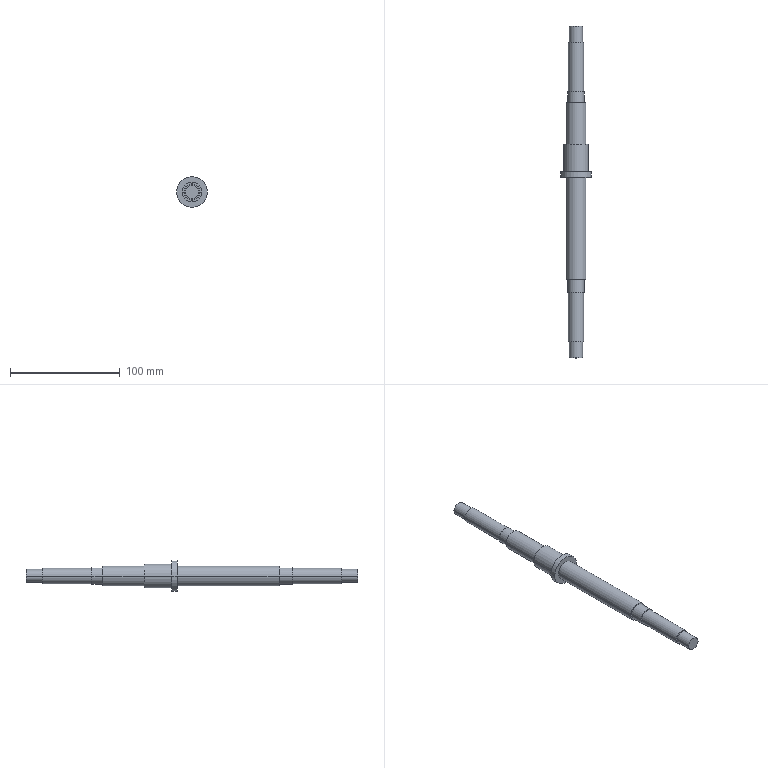Part | SolidWorks | features Revolution 1 | 1 solid | 31 faces | box 28 x 303 x 28 mm | volume 67053 mm3 | cylinder 20 | plane 11 | commonest cylinder face diameters 12 x4 14 x4 15 x4 18 x4 22 x2 28 x2
STEP:
#1=CARTESIAN_POINT('',(-6.,0.,0.));
#2=VERTEX_POINT('',#1);
#3=CARTESIAN_POINT('',(6.,0.,0.));
#4=VERTEX_POINT('',#3);
#5=CARTESIAN_POINT('',(0.,0.,0.));
#6=DIRECTION('',(0.,1.,0.));
#7=DIRECTION('',(-1.,0.,0.));
#8=AXIS2_PLACEMENT_3D('',#5,#6,#7);
#9=CIRCLE('',#8,6.);
#10=EDGE_CURVE('',#2,#4,#9,.T.);
#11=ORIENTED_EDGE('',*,*,#10,.T.);
#12=CARTESIAN_POINT('',(6.,15.,0.));
#13=VERTEX_POINT('',#12);
#14=CARTESIAN_POINT('',(6.,303.,0.));
#15=DIRECTION('',(0.,1.,0.));
#16=VECTOR('',#15,1000.);
#17=LINE('',#14,#16);
#18=EDGE_CURVE('',#4,#13,#17,.T.);
#19=ORIENTED_EDGE('',*,*,#18,.T.);
#20=CARTESIAN_POINT('',(-6.,15.,0.));
#21=VERTEX_POINT('',#20);
#22=CARTESIAN_POINT('',(0.,15.,0.));
#23=DIRECTION('',(0.,1.,0.));
#24=DIRECTION('',(-1.,0.,0.));
#25=AXIS2_PLACEMENT_3D('',#22,#23,#24);
#26=CIRCLE('',#25,6.);
#27=EDGE_CURVE('',#21,#13,#26,.T.);
#28=ORIENTED_EDGE('',*,*,#27,.F.);
#29=CARTESIAN_POINT('',(-6.,303.,0.));
#30=DIRECTION('',(0.,1.,0.));
#31=VECTOR('',#30,1000.);
#32=LINE('',#29,#31);
#33=EDGE_CURVE('',#2,#21,#32,.T.);
#34=ORIENTED_EDGE('',*,*,#33,.F.);
#35=EDGE_LOOP('',(#11,#19,#28,#34));
#36=FACE_OUTER_BOUND('',#35,.T.);
#37=CARTESIAN_POINT('',(0.,303.,0.));
#38=DIRECTION('',(0.,1.,0.));
#39=DIRECTION('',(-1.,0.,0.));
#40=AXIS2_PLACEMENT_3D('',#37,#38,#39);
#41=CYLINDRICAL_SURFACE('',#40,6.);
#42=ADVANCED_FACE('',(#36),#41,.T.);
#43=CARTESIAN_POINT('',(-7.,15.,0.));
#44=VERTEX_POINT('',#43);
#45=CARTESIAN_POINT('',(7.,15.,0.));
#46=VERTEX_POINT('',#45);
#47=CARTESIAN_POINT('',(0.,15.,0.));
#48=DIRECTION('',(0.,1.,0.));
#49=DIRECTION('',(-1.,0.,0.));
#50=AXIS2_PLACEMENT_3D('',#47,#48,#49);
#51=CIRCLE('',#50,7.);
#52=EDGE_CURVE('',#44,#46,#51,.T.);
#53=ORIENTED_EDGE('',*,*,#52,.T.);
#54=CARTESIAN_POINT('',(7.,60.,0.));
#55=VERTEX_POINT('',#54);
#56=CARTESIAN_POINT('',(7.,303.,0.));
#57=DIRECTION('',(0.,1.,0.));
#58=VECTOR('',#57,1000.);
#59=LINE('',#56,#58);
#60=EDGE_CURVE('',#46,#55,#59,.T.);
#61=ORIENTED_EDGE('',*,*,#60,.T.);
#62=CARTESIAN_POINT('',(-7.,60.,0.));
#63=VERTEX_POINT('',#62);
#64=CARTESIAN_POINT('',(0.,60.,0.));
#65=DIRECTION('',(0.,1.,0.));
#66=DIRECTION('',(-1.,0.,0.));
#67=AXIS2_PLACEMENT_3D('',#64,#65,#66);
#68=CIRCLE('',#67,7.);
#69=EDGE_CURVE('',#63,#55,#68,.T.);
#70=ORIENTED_EDGE('',*,*,#69,.F.);
#71=CARTESIAN_POINT('',(-7.,303.,0.));
#72=DIRECTION('',(0.,1.,0.));
#73=VECTOR('',#72,1000.);
#74=LINE('',#71,#73);
#75=EDGE_CURVE('',#44,#63,#74,.T.);
#76=ORIENTED_EDGE('',*,*,#75,.F.);
#77=EDGE_LOOP('',(#53,#61,#70,#76));
#78=FACE_OUTER_BOUND('',#77,.T.);
#79=CARTESIAN_POINT('',(0.,303.,0.));
#80=DIRECTION('',(0.,1.,0.));
#81=DIRECTION('',(-1.,0.,0.));
#82=AXIS2_PLACEMENT_3D('',#79,#80,#81);
#83=CYLINDRICAL_SURFACE('',#82,7.);
#84=ADVANCED_FACE('',(#78),#83,.T.);
#85=CARTESIAN_POINT('',(-7.5,60.,0.));
#86=VERTEX_POINT('',#85);
#87=CARTESIAN_POINT('',(7.5,60.,0.));
#88=VERTEX_POINT('',#87);
#89=CARTESIAN_POINT('',(0.,60.,0.));
#90=DIRECTION('',(0.,1.,0.));
#91=DIRECTION('',(-1.,0.,0.));
#92=AXIS2_PLACEMENT_3D('',#89,#90,#91);
#93=CIRCLE('',#92,7.5);
#94=EDGE_CURVE('',#86,#88,#93,.T.);
#95=ORIENTED_EDGE('',*,*,#94,.T.);
#96=CARTESIAN_POINT('',(7.5,72.,0.));
#97=VERTEX_POINT('',#96);
#98=CARTESIAN_POINT('',(7.5,303.,0.));
#99=DIRECTION('',(0.,1.,0.));
#100=VECTOR('',#99,1000.);
#101=LINE('',#98,#100);
#102=EDGE_CURVE('',#88,#97,#101,.T.);
#103=ORIENTED_EDGE('',*,*,#102,.T.);
#104=CARTESIAN_POINT('',(-7.5,72.,0.));
#105=VERTEX_POINT('',#104);
#106=CARTESIAN_POINT('',(0.,72.,0.));
#107=DIRECTION('',(0.,1.,0.));
#108=DIRECTION('',(-1.,0.,0.));
#109=AXIS2_PLACEMENT_3D('',#106,#107,#108);
#110=CIRCLE('',#109,7.5);
#111=EDGE_CURVE('',#105,#97,#110,.T.);
#112=ORIENTED_EDGE('',*,*,#111,.F.);
#113=CARTESIAN_POINT('',(-7.5,303.,0.));
#114=DIRECTION('',(0.,1.,0.));
#115=VECTOR('',#114,1000.);
#116=LINE('',#113,#115);
#117=EDGE_CURVE('',#86,#105,#116,.T.);
#118=ORIENTED_EDGE('',*,*,#117,.F.);
#119=EDGE_LOOP('',(#95,#103,#112,#118));
#120=FACE_OUTER_BOUND('',#119,.T.);
#121=CARTESIAN_POINT('',(0.,303.,0.));
#122=DIRECTION('',(0.,1.,0.));
#123=DIRECTION('',(-1.,0.,0.));
#124=AXIS2_PLACEMENT_3D('',#121,#122,#123);
#125=CYLINDRICAL_SURFACE('',#124,7.5);
#126=ADVANCED_FACE('',(#120),#125,.T.);
#127=CARTESIAN_POINT('',(-9.,72.,0.));
#128=VERTEX_POINT('',#127);
#129=CARTESIAN_POINT('',(9.,72.,0.));
#130=VERTEX_POINT('',#129);
#131=CARTESIAN_POINT('',(0.,72.,0.));
#132=DIRECTION('',(0.,1.,0.));
#133=DIRECTION('',(-1.,0.,0.));
#134=AXIS2_PLACEMENT_3D('',#131,#132,#133);
#135=CIRCLE('',#134,9.);
#136=EDGE_CURVE('',#128,#130,#135,.T.);
#137=ORIENTED_EDGE('',*,*,#136,.T.);
#138=CARTESIAN_POINT('',(9.,165.,0.));
#139=VERTEX_POINT('',#138);
#140=CARTESIAN_POINT('',(9.,303.,0.));
#141=DIRECTION('',(0.,1.,0.));
#142=VECTOR('',#141,1000.);
#143=LINE('',#140,#142);
#144=EDGE_CURVE('',#130,#139,#143,.T.);
#145=ORIENTED_EDGE('',*,*,#144,.T.);
#146=CARTESIAN_POINT('',(-9.,165.,0.));
#147=VERTEX_POINT('',#146);
#148=CARTESIAN_POINT('',(0.,165.,0.));
#149=DIRECTION('',(0.,1.,0.));
#150=DIRECTION('',(-1.,0.,0.));
#151=AXIS2_PLACEMENT_3D('',#148,#149,#150);
#152=CIRCLE('',#151,9.);
#153=EDGE_CURVE('',#147,#139,#152,.T.);
#154=ORIENTED_EDGE('',*,*,#153,.F.);
#155=CARTESIAN_POINT('',(-9.,303.,0.));
#156=DIRECTION('',(0.,1.,0.));
#157=VECTOR('',#156,1000.);
#158=LINE('',#155,#157);
#159=EDGE_CURVE('',#128,#147,#158,.T.);
#160=ORIENTED_EDGE('',*,*,#159,.F.);
#161=EDGE_LOOP('',(#137,#145,#154,#160));
#162=FACE_OUTER_BOUND('',#161,.T.);
#163=CARTESIAN_POINT('',(0.,303.,0.));
#164=DIRECTION('',(0.,1.,0.));
#165=DIRECTION('',(-1.,0.,0.));
#166=AXIS2_PLACEMENT_3D('',#163,#164,#165);
#167=CYLINDRICAL_SURFACE('',#166,9.);
#168=ADVANCED_FACE('',(#162),#167,.T.);
#169=CARTESIAN_POINT('',(-14.,165.,0.));
#170=VERTEX_POINT('',#169);
#171=CARTESIAN_POINT('',(14.,165.,0.));
#172=VERTEX_POINT('',#171);
#173=CARTESIAN_POINT('',(0.,165.,0.));
#174=DIRECTION('',(0.,1.,0.));
#175=DIRECTION('',(-1.,0.,0.));
#176=AXIS2_PLACEMENT_3D('',#173,#174,#175);
#177=CIRCLE('',#176,14.);
#178=EDGE_CURVE('',#170,#172,#177,.T.);
#179=ORIENTED_EDGE('',*,*,#178,.T.);
#180=CARTESIAN_POINT('',(14.,170.,0.));
#181=VERTEX_POINT('',#180);
#182=CARTESIAN_POINT('',(14.,303.,0.));
#183=DIRECTION('',(0.,1.,0.));
#184=VECTOR('',#183,1000.);
#185=LINE('',#182,#184);
#186=EDGE_CURVE('',#172,#181,#185,.T.);
#187=ORIENTED_EDGE('',*,*,#186,.T.);
#188=CARTESIAN_POINT('',(-14.,170.,0.));
#189=VERTEX_POINT('',#188);
#190=CARTESIAN_POINT('',(0.,170.,0.));
#191=DIRECTION('',(0.,1.,0.));
#192=DIRECTION('',(-1.,0.,0.));
#193=AXIS2_PLACEMENT_3D('',#190,#191,#192);
#194=CIRCLE('',#193,14.);
#195=EDGE_CURVE('',#189,#181,#194,.T.);
#196=ORIENTED_EDGE('',*,*,#195,.F.);
#197=CARTESIAN_POINT('',(-14.,303.,0.));
#198=DIRECTION('',(0.,1.,0.));
#199=VECTOR('',#198,1000.);
#200=LINE('',#197,#199);
#201=EDGE_CURVE('',#170,#189,#200,.T.);
#202=ORIENTED_EDGE('',*,*,#201,.F.);
#203=EDGE_LOOP('',(#179,#187,#196,#202));
#204=FACE_OUTER_BOUND('',#203,.T.);
#205=CARTESIAN_POINT('',(0.,303.,0.));
#206=DIRECTION('',(0.,1.,0.));
#207=DIRECTION('',(-1.,0.,0.));
#208=AXIS2_PLACEMENT_3D('',#205,#206,#207);
#209=CYLINDRICAL_SURFACE('',#208,14.);
#210=ADVANCED_FACE('',(#204),#209,.T.);
#211=CARTESIAN_POINT('',(-11.,170.,0.));
#212=VERTEX_POINT('',#211);
#213=CARTESIAN_POINT('',(11.,170.,0.));
#214=VERTEX_POINT('',#213);
#215=CARTESIAN_POINT('',(0.,170.,0.));
#216=DIRECTION('',(0.,1.,0.));
#217=DIRECTION('',(-1.,0.,0.));
#218=AXIS2_PLACEMENT_3D('',#215,#216,#217);
#219=CIRCLE('',#218,11.);
#220=EDGE_CURVE('',#212,#214,#219,.T.);
#221=ORIENTED_EDGE('',*,*,#220,.T.);
#222=CARTESIAN_POINT('',(11.,195.,0.));
#223=VERTEX_POINT('',#222);
#224=CARTESIAN_POINT('',(11.,303.,0.));
#225=DIRECTION('',(0.,1.,0.));
#226=VECTOR('',#225,1000.);
#227=LINE('',#224,#226);
#228=EDGE_CURVE('',#214,#223,#227,.T.);
#229=ORIENTED_EDGE('',*,*,#228,.T.);
#230=CARTESIAN_POINT('',(-11.,195.,0.));
#231=VERTEX_POINT('',#230);
#232=CARTESIAN_POINT('',(0.,195.,0.));
#233=DIRECTION('',(0.,1.,0.));
#234=DIRECTION('',(-1.,0.,0.));
#235=AXIS2_PLACEMENT_3D('',#232,#233,#234);
#236=CIRCLE('',#235,11.);
#237=EDGE_CURVE('',#231,#223,#236,.T.);
#238=ORIENTED_EDGE('',*,*,#237,.F.);
#239=CARTESIAN_POINT('',(-11.,303.,0.));
#240=DIRECTION('',(0.,1.,0.));
#241=VECTOR('',#240,1000.);
#242=LINE('',#239,#241);
#243=EDGE_CURVE('',#212,#231,#242,.T.);
#244=ORIENTED_EDGE('',*,*,#243,.F.);
#245=EDGE_LOOP('',(#221,#229,#238,#244));
#246=FACE_OUTER_BOUND('',#245,.T.);
#247=CARTESIAN_POINT('',(0.,303.,0.));
#248=DIRECTION('',(0.,1.,0.));
#249=DIRECTION('',(-1.,0.,0.));
#250=AXIS2_PLACEMENT_3D('',#247,#248,#249);
#251=CYLINDRICAL_SURFACE('',#250,11.);
#252=ADVANCED_FACE('',(#246),#251,.T.);
#253=CARTESIAN_POINT('',(-9.,195.,0.));
#254=VERTEX_POINT('',#253);
#255=CARTESIAN_POINT('',(9.,195.,0.));
#256=VERTEX_POINT('',#255);
#257=CARTESIAN_POINT('',(0.,195.,0.));
#258=DIRECTION('',(0.,1.,0.));
#259=DIRECTION('',(-1.,0.,0.));
#260=AXIS2_PLACEMENT_3D('',#257,#258,#259);
#261=CIRCLE('',#260,9.);
#262=EDGE_CURVE('',#254,#256,#261,.T.);
#263=ORIENTED_EDGE('',*,*,#262,.T.);
#264=CARTESIAN_POINT('',(9.,233.,0.));
#265=VERTEX_POINT('',#264);
#266=CARTESIAN_POINT('',(9.,303.,0.));
#267=DIRECTION('',(0.,1.,0.));
#268=VECTOR('',#267,1000.);
#269=LINE('',#266,#268);
#270=EDGE_CURVE('',#256,#265,#269,.T.);
#271=ORIENTED_EDGE('',*,*,#270,.T.);
#272=CARTESIAN_POINT('',(-9.,233.,0.));
#273=VERTEX_POINT('',#272);
#274=CARTESIAN_POINT('',(0.,233.,0.));
#275=DIRECTION('',(0.,1.,0.));
#276=DIRECTION('',(-1.,0.,0.));
#277=AXIS2_PLACEMENT_3D('',#274,#275,#276);
#278=CIRCLE('',#277,9.);
#279=EDGE_CURVE('',#273,#265,#278,.T.);
#280=ORIENTED_EDGE('',*,*,#279,.F.);
#281=CARTESIAN_POINT('',(-9.,303.,0.));
#282=DIRECTION('',(0.,1.,0.));
#283=VECTOR('',#282,1000.);
#284=LINE('',#281,#283);
#285=EDGE_CURVE('',#254,#273,#284,.T.);
#286=ORIENTED_EDGE('',*,*,#285,.F.);
#287=EDGE_LOOP('',(#263,#271,#280,#286));
#288=FACE_OUTER_BOUND('',#287,.T.);
#289=CARTESIAN_POINT('',(0.,303.,0.));
#290=DIRECTION('',(0.,1.,0.));
#291=DIRECTION('',(-1.,0.,0.));
#292=AXIS2_PLACEMENT_3D('',#289,#290,#291);
#293=CYLINDRICAL_SURFACE('',#292,9.);
#294=ADVANCED_FACE('',(#288),#293,.T.);
#295=CARTESIAN_POINT('',(-7.5,233.,0.));
#296=VERTEX_POINT('',#295);
#297=CARTESIAN_POINT('',(7.5,233.,0.));
#298=VERTEX_POINT('',#297);
#299=CARTESIAN_POINT('',(0.,233.,0.));
#300=DIRECTION('',(0.,1.,0.));
#301=DIRECTION('',(-1.,0.,0.));
#302=AXIS2_PLACEMENT_3D('',#299,#300,#301);
#303=CIRCLE('',#302,7.5);
#304=EDGE_CURVE('',#296,#298,#303,.T.);
#305=ORIENTED_EDGE('',*,*,#304,.T.);
#306=CARTESIAN_POINT('',(7.5,243.,0.));
#307=VERTEX_POINT('',#306);
#308=CARTESIAN_POINT('',(7.5,303.,0.));
#309=DIRECTION('',(0.,1.,0.));
#310=VECTOR('',#309,1000.);
#311=LINE('',#308,#310);
#312=EDGE_CURVE('',#298,#307,#311,.T.);
#313=ORIENTED_EDGE('',*,*,#312,.T.);
#314=CARTESIAN_POINT('',(-7.5,243.,0.));
#315=VERTEX_POINT('',#314);
#316=CARTESIAN_POINT('',(0.,243.,0.));
#317=DIRECTION('',(0.,1.,0.));
#318=DIRECTION('',(-1.,0.,0.));
#319=AXIS2_PLACEMENT_3D('',#316,#317,#318);
#320=CIRCLE('',#319,7.5);
#321=EDGE_CURVE('',#315,#307,#320,.T.);
#322=ORIENTED_EDGE('',*,*,#321,.F.);
#323=CARTESIAN_POINT('',(-7.5,303.,0.));
#324=DIRECTION('',(0.,1.,0.));
#325=VECTOR('',#324,1000.);
#326=LINE('',#323,#325);
#327=EDGE_CURVE('',#296,#315,#326,.T.);
#328=ORIENTED_EDGE('',*,*,#327,.F.);
#329=EDGE_LOOP('',(#305,#313,#322,#328));
#330=FACE_OUTER_BOUND('',#329,.T.);
#331=CARTESIAN_POINT('',(0.,303.,0.));
#332=DIRECTION('',(0.,1.,0.));
#333=DIRECTION('',(-1.,0.,0.));
#334=AXIS2_PLACEMENT_3D('',#331,#332,#333);
#335=CYLINDRICAL_SURFACE('',#334,7.5);
#336=ADVANCED_FACE('',(#330),#335,.T.);
#337=CARTESIAN_POINT('',(-7.,243.,0.));
#338=VERTEX_POINT('',#337);
#339=CARTESIAN_POINT('',(7.,243.,0.));
#340=VERTEX_POINT('',#339);
#341=CARTESIAN_POINT('',(0.,243.,0.));
#342=DIRECTION('',(0.,1.,0.));
#343=DIRECTION('',(-1.,0.,0.));
#344=AXIS2_PLACEMENT_3D('',#341,#342,#343);
#345=CIRCLE('',#344,7.);
#346=EDGE_CURVE('',#338,#340,#345,.T.);
#347=ORIENTED_EDGE('',*,*,#346,.T.);
#348=CARTESIAN_POINT('',(7.,288.,0.));
#349=VERTEX_POINT('',#348);
#350=CARTESIAN_POINT('',(7.,303.,0.));
#351=DIRECTION('',(0.,1.,0.));
#352=VECTOR('',#351,1000.);
#353=LINE('',#350,#352);
#354=EDGE_CURVE('',#340,#349,#353,.T.);
#355=ORIENTED_EDGE('',*,*,#354,.T.);
#356=CARTESIAN_POINT('',(-7.,288.,0.));
#357=VERTEX_POINT('',#356);
#358=CARTESIAN_POINT('',(0.,288.,0.));
#359=DIRECTION('',(0.,1.,0.));
#360=DIRECTION('',(-1.,0.,0.));
#361=AXIS2_PLACEMENT_3D('',#358,#359,#360);
#362=CIRCLE('',#361,7.);
#363=EDGE_CURVE('',#357,#349,#362,.T.);
#364=ORIENTED_EDGE('',*,*,#363,.F.);
#365=CARTESIAN_POINT('',(-7.,303.,0.));
#366=DIRECTION('',(0.,1.,0.));
#367=VECTOR('',#366,1000.);
#368=LINE('',#365,#367);
#369=EDGE_CURVE('',#338,#357,#368,.T.);
#370=ORIENTED_EDGE('',*,*,#369,.F.);
#371=EDGE_LOOP('',(#347,#355,#364,#370));
#372=FACE_OUTER_BOUND('',#371,.T.);
#373=CARTESIAN_POINT('',(0.,303.,0.));
#374=DIRECTION('',(0.,1.,0.));
#375=DIRECTION('',(-1.,0.,0.));
#376=AXIS2_PLACEMENT_3D('',#373,#374,#375);
#377=CYLINDRICAL_SURFACE('',#376,7.);
#378=ADVANCED_FACE('',(#372),#377,.T.);
#379=CARTESIAN_POINT('',(-6.,288.,0.));
#380=VERTEX_POINT('',#379);
#381=CARTESIAN_POINT('',(6.,288.,0.));
#382=VERTEX_POINT('',#381);
#383=CARTESIAN_POINT('',(0.,288.,0.));
#384=DIRECTION('',(0.,1.,0.));
#385=DIRECTION('',(-1.,0.,0.));
#386=AXIS2_PLACEMENT_3D('',#383,#384,#385);
#387=CIRCLE('',#386,6.);
#388=EDGE_CURVE('',#380,#382,#387,.T.);
#389=ORIENTED_EDGE('',*,*,#388,.T.);
#390=CARTESIAN_POINT('',(6.,303.,0.));
#391=VERTEX_POINT('',#390);
#392=CARTESIAN_POINT('',(6.,303.,0.));
#393=DIRECTION('',(0.,1.,0.));
#394=VECTOR('',#393,1000.);
#395=LINE('',#392,#394);
#396=EDGE_CURVE('',#382,#391,#395,.T.);
#397=ORIENTED_EDGE('',*,*,#396,.T.);
#398=CARTESIAN_POINT('',(-6.,303.,0.));
#399=VERTEX_POINT('',#398);
#400=CARTESIAN_POINT('',(0.,303.,0.));
#401=DIRECTION('',(0.,1.,0.));
#402=DIRECTION('',(-1.,0.,0.));
#403=AXIS2_PLACEMENT_3D('',#400,#401,#402);
#404=CIRCLE('',#403,6.);
#405=EDGE_CURVE('',#399,#391,#404,.T.);
#406=ORIENTED_EDGE('',*,*,#405,.F.);
#407=CARTESIAN_POINT('',(-6.,303.,0.));
#408=DIRECTION('',(0.,1.,0.));
#409=VECTOR('',#408,1000.);
#410=LINE('',#407,#409);
#411=EDGE_CURVE('',#380,#399,#410,.T.);
#412=ORIENTED_EDGE('',*,*,#411,.F.);
#413=EDGE_LOOP('',(#389,#397,#406,#412));
#414=FACE_OUTER_BOUND('',#413,.T.);
#415=CARTESIAN_POINT('',(0.,303.,0.));
#416=DIRECTION('',(0.,1.,0.));
#417=DIRECTION('',(-1.,0.,0.));
#418=AXIS2_PLACEMENT_3D('',#415,#416,#417);
#419=CYLINDRICAL_SURFACE('',#418,6.);
#420=ADVANCED_FACE('',(#414),#419,.T.);
#421=ORIENTED_EDGE('',*,*,#405,.T.);
#422=CARTESIAN_POINT('',(0.,303.,0.));
#423=DIRECTION('',(0.,1.,0.));
#424=DIRECTION('',(-1.,0.,0.));
#425=AXIS2_PLACEMENT_3D('',#422,#423,#424);
#426=CIRCLE('',#425,6.);
#427=EDGE_CURVE('',#391,#399,#426,.T.);
#428=ORIENTED_EDGE('',*,*,#427,.T.);
#429=EDGE_LOOP('',(#421,#428));
#430=FACE_OUTER_BOUND('',#429,.T.);
#431=CARTESIAN_POINT('',(0.,303.,0.));
#432=DIRECTION('',(0.,1.,0.));
#433=DIRECTION('',(-1.,0.,0.));
#434=AXIS2_PLACEMENT_3D('',#431,#432,#433);
#435=PLANE('',#434);
#436=ADVANCED_FACE('',(#430),#435,.T.);
#437=ORIENTED_EDGE('',*,*,#396,.F.);
#438=CARTESIAN_POINT('',(0.,288.,0.));
#439=DIRECTION('',(0.,1.,0.));
#440=DIRECTION('',(-1.,0.,0.));
#441=AXIS2_PLACEMENT_3D('',#438,#439,#440);
#442=CIRCLE('',#441,6.);
#443=EDGE_CURVE('',#382,#380,#442,.T.);
#444=ORIENTED_EDGE('',*,*,#443,.T.);
#445=ORIENTED_EDGE('',*,*,#411,.T.);
#446=ORIENTED_EDGE('',*,*,#427,.F.);
#447=EDGE_LOOP('',(#437,#444,#445,#446));
#448=FACE_OUTER_BOUND('',#447,.T.);
#449=CARTESIAN_POINT('',(0.,303.,0.));
#450=DIRECTION('',(0.,1.,0.));
#451=DIRECTION('',(-1.,0.,0.));
#452=AXIS2_PLACEMENT_3D('',#449,#450,#451);
#453=CYLINDRICAL_SURFACE('',#452,6.);
#454=ADVANCED_FACE('',(#448),#453,.T.);
#455=ORIENTED_EDGE('',*,*,#363,.T.);
#456=CARTESIAN_POINT('',(0.,288.,0.));
#457=DIRECTION('',(0.,1.,0.));
#458=DIRECTION('',(-1.,0.,0.));
#459=AXIS2_PLACEMENT_3D('',#456,#457,#458);
#460=CIRCLE('',#459,7.);
#461=EDGE_CURVE('',#349,#357,#460,.T.);
#462=ORIENTED_EDGE('',*,*,#461,.T.);
#463=EDGE_LOOP('',(#455,#462));
#464=FACE_OUTER_BOUND('',#463,.T.);
#465=ORIENTED_EDGE('',*,*,#388,.F.);
#466=ORIENTED_EDGE('',*,*,#443,.F.);
#467=EDGE_LOOP('',(#465,#466));
#468=FACE_BOUND('',#467,.T.);
#469=CARTESIAN_POINT('',(-6.,288.,0.));
#470=DIRECTION('',(0.,1.,0.));
#471=DIRECTION('',(-1.,0.,0.));
#472=AXIS2_PLACEMENT_3D('',#469,#470,#471);
#473=PLANE('',#472);
#474=ADVANCED_FACE('',(#464,#468),#473,.T.);
#475=ORIENTED_EDGE('',*,*,#354,.F.);
#476=CARTESIAN_POINT('',(0.,243.,0.));
#477=DIRECTION('',(0.,1.,0.));
#478=DIRECTION('',(-1.,0.,0.));
#479=AXIS2_PLACEMENT_3D('',#476,#477,#478);
#480=CIRCLE('',#479,7.);
#481=EDGE_CURVE('',#340,#338,#480,.T.);
#482=ORIENTED_EDGE('',*,*,#481,.T.);
#483=ORIENTED_EDGE('',*,*,#369,.T.);
#484=ORIENTED_EDGE('',*,*,#461,.F.);
#485=EDGE_LOOP('',(#475,#482,#483,#484));
#486=FACE_OUTER_BOUND('',#485,.T.);
#487=CARTESIAN_POINT('',(0.,303.,0.));
#488=DIRECTION('',(0.,1.,0.));
#489=DIRECTION('',(-1.,0.,0.));
#490=AXIS2_PLACEMENT_3D('',#487,#488,#489);
#491=CYLINDRICAL_SURFACE('',#490,7.);
#492=ADVANCED_FACE('',(#486),#491,.T.);
#493=ORIENTED_EDGE('',*,*,#321,.T.);
#494=CARTESIAN_POINT('',(0.,243.,0.));
#495=DIRECTION('',(0.,1.,0.));
#496=DIRECTION('',(-1.,0.,0.));
#497=AXIS2_PLACEMENT_3D('',#494,#495,#496);
#498=CIRCLE('',#497,7.5);
#499=EDGE_CURVE('',#307,#315,#498,.T.);
#500=ORIENTED_EDGE('',*,*,#499,.T.);
#501=EDGE_LOOP('',(#493,#500));
#502=FACE_OUTER_BOUND('',#501,.T.);
#503=ORIENTED_EDGE('',*,*,#346,.F.);
#504=ORIENTED_EDGE('',*,*,#481,.F.);
#505=EDGE_LOOP('',(#503,#504));
#506=FACE_BOUND('',#505,.T.);
#507=CARTESIAN_POINT('',(-7.,243.,0.));
#508=DIRECTION('',(0.,1.,0.));
#509=DIRECTION('',(-1.,0.,0.));
#510=AXIS2_PLACEMENT_3D('',#507,#508,#509);
#511=PLANE('',#510);
#512=ADVANCED_FACE('',(#502,#506),#511,.T.);
#513=ORIENTED_EDGE('',*,*,#312,.F.);
#514=CARTESIAN_POINT('',(0.,233.,0.));
#515=DIRECTION('',(0.,1.,0.));
#516=DIRECTION('',(-1.,0.,0.));
#517=AXIS2_PLACEMENT_3D('',#514,#515,#516);
#518=CIRCLE('',#517,7.5);
#519=EDGE_CURVE('',#298,#296,#518,.T.);
#520=ORIENTED_EDGE('',*,*,#519,.T.);
#521=ORIENTED_EDGE('',*,*,#327,.T.);
#522=ORIENTED_EDGE('',*,*,#499,.F.);
#523=EDGE_LOOP('',(#513,#520,#521,#522));
#524=FACE_OUTER_BOUND('',#523,.T.);
#525=CARTESIAN_POINT('',(0.,303.,0.));
#526=DIRECTION('',(0.,1.,0.));
#527=DIRECTION('',(-1.,0.,0.));
#528=AXIS2_PLACEMENT_3D('',#525,#526,#527);
#529=CYLINDRICAL_SURFACE('',#528,7.5);
#530=ADVANCED_FACE('',(#524),#529,.T.);
#531=ORIENTED_EDGE('',*,*,#279,.T.);
#532=CARTESIAN_POINT('',(0.,233.,0.));
#533=DIRECTION('',(0.,1.,0.));
#534=DIRECTION('',(-1.,0.,0.));
#535=AXIS2_PLACEMENT_3D('',#532,#533,#534);
#536=CIRCLE('',#535,9.);
#537=EDGE_CURVE('',#265,#273,#536,.T.);
#538=ORIENTED_EDGE('',*,*,#537,.T.);
#539=EDGE_LOOP('',(#531,#538));
#540=FACE_OUTER_BOUND('',#539,.T.);
#541=ORIENTED_EDGE('',*,*,#304,.F.);
#542=ORIENTED_EDGE('',*,*,#519,.F.);
#543=EDGE_LOOP('',(#541,#542));
#544=FACE_BOUND('',#543,.T.);
#545=CARTESIAN_POINT('',(-7.5,233.,0.));
#546=DIRECTION('',(0.,1.,0.));
#547=DIRECTION('',(-1.,0.,0.));
#548=AXIS2_PLACEMENT_3D('',#545,#546,#547);
#549=PLANE('',#548);
#550=ADVANCED_FACE('',(#540,#544),#549,.T.);
#551=ORIENTED_EDGE('',*,*,#270,.F.);
#552=CARTESIAN_POINT('',(0.,195.,0.));
#553=DIRECTION('',(0.,1.,0.));
#554=DIRECTION('',(-1.,0.,0.));
#555=AXIS2_PLACEMENT_3D('',#552,#553,#554);
#556=CIRCLE('',#555,9.);
#557=EDGE_CURVE('',#256,#254,#556,.T.);
#558=ORIENTED_EDGE('',*,*,#557,.T.);
#559=ORIENTED_EDGE('',*,*,#285,.T.);
#560=ORIENTED_EDGE('',*,*,#537,.F.);
#561=EDGE_LOOP('',(#551,#558,#559,#560));
#562=FACE_OUTER_BOUND('',#561,.T.);
#563=CARTESIAN_POINT('',(0.,303.,0.));
#564=DIRECTION('',(0.,1.,0.));
#565=DIRECTION('',(-1.,0.,0.));
#566=AXIS2_PLACEMENT_3D('',#563,#564,#565);
#567=CYLINDRICAL_SURFACE('',#566,9.);
#568=ADVANCED_FACE('',(#562),#567,.T.);
#569=ORIENTED_EDGE('',*,*,#237,.T.);
#570=CARTESIAN_POINT('',(0.,195.,0.));
#571=DIRECTION('',(0.,1.,0.));
#572=DIRECTION('',(-1.,0.,0.));
#573=AXIS2_PLACEMENT_3D('',#570,#571,#572);
#574=CIRCLE('',#573,11.);
#575=EDGE_CURVE('',#223,#231,#574,.T.);
#576=ORIENTED_EDGE('',*,*,#575,.T.);
#577=EDGE_LOOP('',(#569,#576));
#578=FACE_OUTER_BOUND('',#577,.T.);
#579=ORIENTED_EDGE('',*,*,#262,.F.);
#580=ORIENTED_EDGE('',*,*,#557,.F.);
#581=EDGE_LOOP('',(#579,#580));
#582=FACE_BOUND('',#581,.T.);
#583=CARTESIAN_POINT('',(-9.,195.,0.));
#584=DIRECTION('',(0.,1.,0.));
#585=DIRECTION('',(-1.,0.,0.));
#586=AXIS2_PLACEMENT_3D('',#583,#584,#585);
#587=PLANE('',#586);
#588=ADVANCED_FACE('',(#578,#582),#587,.T.);
#589=ORIENTED_EDGE('',*,*,#228,.F.);
#590=CARTESIAN_POINT('',(0.,170.,0.));
#591=DIRECTION('',(0.,1.,0.));
#592=DIRECTION('',(-1.,0.,0.));
#593=AXIS2_PLACEMENT_3D('',#590,#591,#592);
#594=CIRCLE('',#593,11.);
#595=EDGE_CURVE('',#214,#212,#594,.T.);
#596=ORIENTED_EDGE('',*,*,#595,.T.);
#597=ORIENTED_EDGE('',*,*,#243,.T.);
#598=ORIENTED_EDGE('',*,*,#575,.F.);
#599=EDGE_LOOP('',(#589,#596,#597,#598));
#600=FACE_OUTER_BOUND('',#599,.T.);
#601=CARTESIAN_POINT('',(0.,303.,0.));
#602=DIRECTION('',(0.,1.,0.));
#603=DIRECTION('',(-1.,0.,0.));
#604=AXIS2_PLACEMENT_3D('',#601,#602,#603);
#605=CYLINDRICAL_SURFACE('',#604,11.);
#606=ADVANCED_FACE('',(#600),#605,.T.);
#607=ORIENTED_EDGE('',*,*,#195,.T.);
#608=CARTESIAN_POINT('',(0.,170.,0.));
#609=DIRECTION('',(0.,1.,0.));
#610=DIRECTION('',(-1.,0.,0.));
#611=AXIS2_PLACEMENT_3D('',#608,#609,#610);
#612=CIRCLE('',#611,14.);
#613=EDGE_CURVE('',#181,#189,#612,.T.);
#614=ORIENTED_EDGE('',*,*,#613,.T.);
#615=EDGE_LOOP('',(#607,#614));
#616=FACE_OUTER_BOUND('',#615,.T.);
#617=ORIENTED_EDGE('',*,*,#220,.F.);
#618=ORIENTED_EDGE('',*,*,#595,.F.);
#619=EDGE_LOOP('',(#617,#618));
#620=FACE_BOUND('',#619,.T.);
#621=CARTESIAN_POINT('',(-11.,170.,0.));
#622=DIRECTION('',(0.,1.,0.));
#623=DIRECTION('',(-1.,0.,0.));
#624=AXIS2_PLACEMENT_3D('',#621,#622,#623);
#625=PLANE('',#624);
#626=ADVANCED_FACE('',(#616,#620),#625,.T.);
#627=ORIENTED_EDGE('',*,*,#186,.F.);
#628=CARTESIAN_POINT('',(0.,165.,0.));
#629=DIRECTION('',(0.,1.,0.));
#630=DIRECTION('',(-1.,0.,0.));
#631=AXIS2_PLACEMENT_3D('',#628,#629,#630);
#632=CIRCLE('',#631,14.);
#633=EDGE_CURVE('',#172,#170,#632,.T.);
#634=ORIENTED_EDGE('',*,*,#633,.T.);
#635=ORIENTED_EDGE('',*,*,#201,.T.);
#636=ORIENTED_EDGE('',*,*,#613,.F.);
#637=EDGE_LOOP('',(#627,#634,#635,#636));
#638=FACE_OUTER_BOUND('',#637,.T.);
#639=CARTESIAN_POINT('',(0.,303.,0.));
#640=DIRECTION('',(0.,1.,0.));
#641=DIRECTION('',(-1.,0.,0.));
#642=AXIS2_PLACEMENT_3D('',#639,#640,#641);
#643=CYLINDRICAL_SURFACE('',#642,14.);
#644=ADVANCED_FACE('',(#638),#643,.T.);
#645=ORIENTED_EDGE('',*,*,#153,.T.);
#646=CARTESIAN_POINT('',(0.,165.,0.));
#647=DIRECTION('',(0.,1.,0.));
#648=DIRECTION('',(-1.,0.,0.));
#649=AXIS2_PLACEMENT_3D('',#646,#647,#648);
#650=CIRCLE('',#649,9.);
#651=EDGE_CURVE('',#139,#147,#650,.T.);
#652=ORIENTED_EDGE('',*,*,#651,.T.);
#653=EDGE_LOOP('',(#645,#652));
#654=FACE_BOUND('',#653,.T.);
#655=ORIENTED_EDGE('',*,*,#178,.F.);
#656=ORIENTED_EDGE('',*,*,#633,.F.);
#657=EDGE_LOOP('',(#655,#656));
#658=FACE_OUTER_BOUND('',#657,.T.);
#659=CARTESIAN_POINT('',(-14.,165.,0.));
#660=DIRECTION('',(0.,-1.,0.));
#661=DIRECTION('',(1.,0.,0.));
#662=AXIS2_PLACEMENT_3D('',#659,#660,#661);
#663=PLANE('',#662);
#664=ADVANCED_FACE('',(#654,#658),#663,.T.);
#665=ORIENTED_EDGE('',*,*,#144,.F.);
#666=CARTESIAN_POINT('',(0.,72.,0.));
#667=DIRECTION('',(0.,1.,0.));
#668=DIRECTION('',(-1.,0.,0.));
#669=AXIS2_PLACEMENT_3D('',#666,#667,#668);
#670=CIRCLE('',#669,9.);
#671=EDGE_CURVE('',#130,#128,#670,.T.);
#672=ORIENTED_EDGE('',*,*,#671,.T.);
#673=ORIENTED_EDGE('',*,*,#159,.T.);
#674=ORIENTED_EDGE('',*,*,#651,.F.);
#675=EDGE_LOOP('',(#665,#672,#673,#674));
#676=FACE_OUTER_BOUND('',#675,.T.);
#677=CARTESIAN_POINT('',(0.,303.,0.));
#678=DIRECTION('',(0.,1.,0.));
#679=DIRECTION('',(-1.,0.,0.));
#680=AXIS2_PLACEMENT_3D('',#677,#678,#679);
#681=CYLINDRICAL_SURFACE('',#680,9.);
#682=ADVANCED_FACE('',(#676),#681,.T.);
#683=ORIENTED_EDGE('',*,*,#111,.T.);
#684=CARTESIAN_POINT('',(0.,72.,0.));
#685=DIRECTION('',(0.,1.,0.));
#686=DIRECTION('',(-1.,0.,0.));
#687=AXIS2_PLACEMENT_3D('',#684,#685,#686);
#688=CIRCLE('',#687,7.5);
#689=EDGE_CURVE('',#97,#105,#688,.T.);
#690=ORIENTED_EDGE('',*,*,#689,.T.);
#691=EDGE_LOOP('',(#683,#690));
#692=FACE_BOUND('',#691,.T.);
#693=ORIENTED_EDGE('',*,*,#136,.F.);
#694=ORIENTED_EDGE('',*,*,#671,.F.);
#695=EDGE_LOOP('',(#693,#694));
#696=FACE_OUTER_BOUND('',#695,.T.);
#697=CARTESIAN_POINT('',(-9.,72.,0.));
#698=DIRECTION('',(0.,-1.,0.));
#699=DIRECTION('',(1.,0.,0.));
#700=AXIS2_PLACEMENT_3D('',#697,#698,#699);
#701=PLANE('',#700);
#702=ADVANCED_FACE('',(#692,#696),#701,.T.);
#703=ORIENTED_EDGE('',*,*,#102,.F.);
#704=CARTESIAN_POINT('',(0.,60.,0.));
#705=DIRECTION('',(0.,1.,0.));
#706=DIRECTION('',(-1.,0.,0.));
#707=AXIS2_PLACEMENT_3D('',#704,#705,#706);
#708=CIRCLE('',#707,7.5);
#709=EDGE_CURVE('',#88,#86,#708,.T.);
#710=ORIENTED_EDGE('',*,*,#709,.T.);
#711=ORIENTED_EDGE('',*,*,#117,.T.);
#712=ORIENTED_EDGE('',*,*,#689,.F.);
#713=EDGE_LOOP('',(#703,#710,#711,#712));
#714=FACE_OUTER_BOUND('',#713,.T.);
#715=CARTESIAN_POINT('',(0.,303.,0.));
#716=DIRECTION('',(0.,1.,0.));
#717=DIRECTION('',(-1.,0.,0.));
#718=AXIS2_PLACEMENT_3D('',#715,#716,#717);
#719=CYLINDRICAL_SURFACE('',#718,7.5);
#720=ADVANCED_FACE('',(#714),#719,.T.);
#721=ORIENTED_EDGE('',*,*,#69,.T.);
#722=CARTESIAN_POINT('',(0.,60.,0.));
#723=DIRECTION('',(0.,1.,0.));
#724=DIRECTION('',(-1.,0.,0.));
#725=AXIS2_PLACEMENT_3D('',#722,#723,#724);
#726=CIRCLE('',#725,7.);
#727=EDGE_CURVE('',#55,#63,#726,.T.);
#728=ORIENTED_EDGE('',*,*,#727,.T.);
#729=EDGE_LOOP('',(#721,#728));
#730=FACE_BOUND('',#729,.T.);
#731=ORIENTED_EDGE('',*,*,#94,.F.);
#732=ORIENTED_EDGE('',*,*,#709,.F.);
#733=EDGE_LOOP('',(#731,#732));
#734=FACE_OUTER_BOUND('',#733,.T.);
#735=CARTESIAN_POINT('',(-7.5,60.,0.));
#736=DIRECTION('',(0.,-1.,0.));
#737=DIRECTION('',(1.,0.,0.));
#738=AXIS2_PLACEMENT_3D('',#735,#736,#737);
#739=PLANE('',#738);
#740=ADVANCED_FACE('',(#730,#734),#739,.T.);
#741=ORIENTED_EDGE('',*,*,#60,.F.);
#742=CARTESIAN_POINT('',(0.,15.,0.));
#743=DIRECTION('',(0.,1.,0.));
#744=DIRECTION('',(-1.,0.,0.));
#745=AXIS2_PLACEMENT_3D('',#742,#743,#744);
#746=CIRCLE('',#745,7.);
#747=EDGE_CURVE('',#46,#44,#746,.T.);
#748=ORIENTED_EDGE('',*,*,#747,.T.);
#749=ORIENTED_EDGE('',*,*,#75,.T.);
#750=ORIENTED_EDGE('',*,*,#727,.F.);
#751=EDGE_LOOP('',(#741,#748,#749,#750));
#752=FACE_OUTER_BOUND('',#751,.T.);
#753=CARTESIAN_POINT('',(0.,303.,0.));
#754=DIRECTION('',(0.,1.,0.));
#755=DIRECTION('',(-1.,0.,0.));
#756=AXIS2_PLACEMENT_3D('',#753,#754,#755);
#757=CYLINDRICAL_SURFACE('',#756,7.);
#758=ADVANCED_FACE('',(#752),#757,.T.);
#759=ORIENTED_EDGE('',*,*,#27,.T.);
#760=CARTESIAN_POINT('',(0.,15.,0.));
#761=DIRECTION('',(0.,1.,0.));
#762=DIRECTION('',(-1.,0.,0.));
#763=AXIS2_PLACEMENT_3D('',#760,#761,#762);
#764=CIRCLE('',#763,6.);
#765=EDGE_CURVE('',#13,#21,#764,.T.);
#766=ORIENTED_EDGE('',*,*,#765,.T.);
#767=EDGE_LOOP('',(#759,#766));
#768=FACE_BOUND('',#767,.T.);
#769=ORIENTED_EDGE('',*,*,#52,.F.);
#770=ORIENTED_EDGE('',*,*,#747,.F.);
#771=EDGE_LOOP('',(#769,#770));
#772=FACE_OUTER_BOUND('',#771,.T.);
#773=CARTESIAN_POINT('',(-7.,15.,0.));
#774=DIRECTION('',(0.,-1.,0.));
#775=DIRECTION('',(1.,0.,0.));
#776=AXIS2_PLACEMENT_3D('',#773,#774,#775);
#777=PLANE('',#776);
#778=ADVANCED_FACE('',(#768,#772),#777,.T.);
#779=ORIENTED_EDGE('',*,*,#18,.F.);
#780=CARTESIAN_POINT('',(0.,0.,0.));
#781=DIRECTION('',(0.,1.,0.));
#782=DIRECTION('',(-1.,0.,0.));
#783=AXIS2_PLACEMENT_3D('',#780,#781,#782);
#784=CIRCLE('',#783,6.);
#785=EDGE_CURVE('',#4,#2,#784,.T.);
#786=ORIENTED_EDGE('',*,*,#785,.T.);
#787=ORIENTED_EDGE('',*,*,#33,.T.);
#788=ORIENTED_EDGE('',*,*,#765,.F.);
#789=EDGE_LOOP('',(#779,#786,#787,#788));
#790=FACE_OUTER_BOUND('',#789,.T.);
#791=CARTESIAN_POINT('',(0.,303.,0.));
#792=DIRECTION('',(0.,1.,0.));
#793=DIRECTION('',(-1.,0.,0.));
#794=AXIS2_PLACEMENT_3D('',#791,#792,#793);
#795=CYLINDRICAL_SURFACE('',#794,6.);
#796=ADVANCED_FACE('',(#790),#795,.T.);
#797=ORIENTED_EDGE('',*,*,#10,.F.);
#798=ORIENTED_EDGE('',*,*,#785,.F.);
#799=EDGE_LOOP('',(#797,#798));
#800=FACE_OUTER_BOUND('',#799,.T.);
#801=CARTESIAN_POINT('',(-6.,0.,0.));
#802=DIRECTION('',(0.,-1.,0.));
#803=DIRECTION('',(1.,0.,0.));
#804=AXIS2_PLACEMENT_3D('',#801,#802,#803);
#805=PLANE('',#804);
#806=ADVANCED_FACE('',(#800),#805,.T.);
#807=CLOSED_SHELL('',(#42,#84,#126,#168,#210,#252,#294,#336,#378,#420,#436,#454,#474,#492,#512,#530,#550,#568,#588,#606,#626,#644,#664,#682,#702,#720,#740,#758,#778,#796,#806));
#808=MANIFOLD_SOLID_BREP('',#807);
#809=CARTESIAN_POINT('',(0.,0.,0.));
#810=DIRECTION('',(0.,0.,1.));
#811=DIRECTION('',(1.,0.,0.));
#812=AXIS2_PLACEMENT_3D('',#809,#810,#811);
#813=(LENGTH_UNIT()NAMED_UNIT(*)SI_UNIT(.MILLI.,.METRE.));
#814=UNCERTAINTY_MEASURE_WITH_UNIT(LENGTH_MEASURE(0.00001),#813,'','');
#815=(NAMED_UNIT(*)PLANE_ANGLE_UNIT()SI_UNIT($,.RADIAN.));
#816=(NAMED_UNIT(*)SI_UNIT($,.STERADIAN.)SOLID_ANGLE_UNIT());
#817=(GEOMETRIC_REPRESENTATION_CONTEXT(3)GLOBAL_UNCERTAINTY_ASSIGNED_CONTEXT((#814))GLOBAL_UNIT_ASSIGNED_CONTEXT((#813,#815,#816))REPRESENTATION_CONTEXT('',''));
#818=ADVANCED_BREP_SHAPE_REPRESENTATION('',(#808,#812),#817);